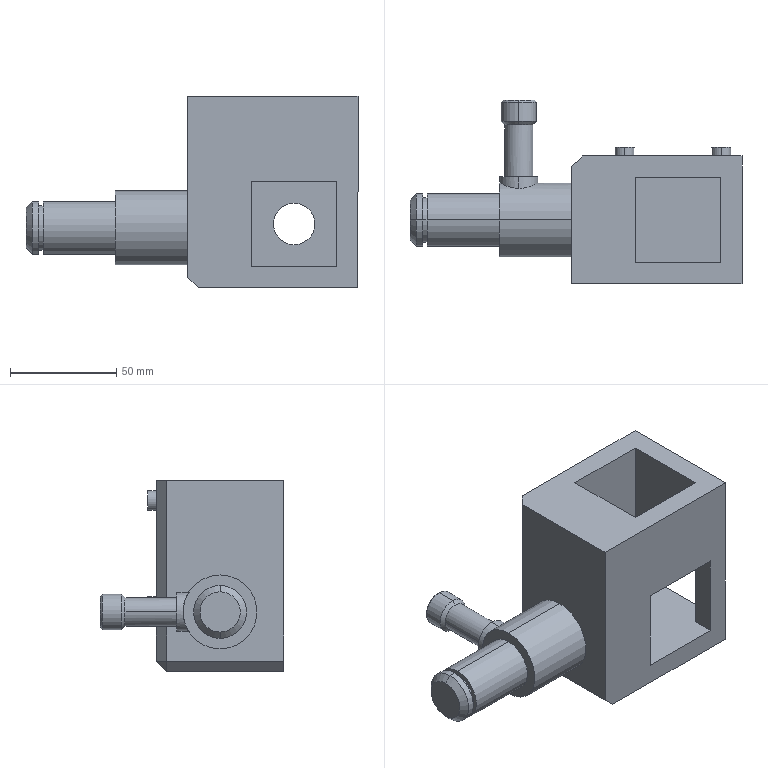Part | SolidWorks | features ICE 13, Chamfer 4, Extrusion 1 | 1 solid | 90 faces | box 156 x 86.375 x 90 mm | volume 325727 mm3 | plane 58 | cylinder 26 | cone 6 | commonest cylinder face diameters 8 x4 9 x4 24.916 x4 9.979 x2 13.306 x2 16.71 x2